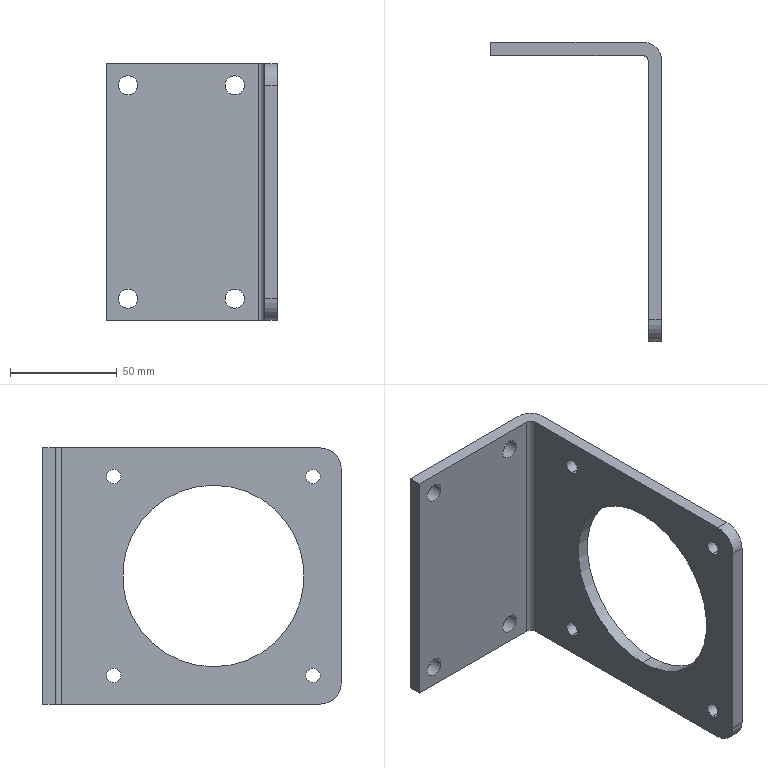Part | STEP file | X77-07004 | 1 solid | 30 faces | box 80 x 140 x 120 mm | volume 115961 mm3 | cylinder 22 | plane 8 | commonest cylinder face diameters 6.8 x8 9 x8 20 x2 85 x2 6 x1 16 x1
STEP:
#1=CARTESIAN_POINT('',(374.189,-142.541,9.95));
#2=VERTEX_POINT('',#1);
#3=CARTESIAN_POINT('',(374.189,-142.541,16.75));
#4=VERTEX_POINT('',#3);
#5=CARTESIAN_POINT('',(374.189,-142.541,13.35));
#6=DIRECTION('',(-1.,0.,0.));
#7=DIRECTION('',(0.,0.,1.));
#8=AXIS2_PLACEMENT_3D('',#5,#6,#7);
#9=CIRCLE('',#8,3.4);
#10=EDGE_CURVE('',#2,#4,#9,.T.);
#11=ORIENTED_EDGE('',*,*,#10,.F.);
#12=CARTESIAN_POINT('',(368.189,-142.541,9.95));
#13=VERTEX_POINT('',#12);
#14=CARTESIAN_POINT('',(368.189,-142.541,9.95));
#15=DIRECTION('',(-1.,0.,0.));
#16=VECTOR('',#15,1000.);
#17=LINE('',#14,#16);
#18=EDGE_CURVE('',#2,#13,#17,.T.);
#19=ORIENTED_EDGE('',*,*,#18,.T.);
#20=CARTESIAN_POINT('',(368.189,-142.541,16.75));
#21=VERTEX_POINT('',#20);
#22=CARTESIAN_POINT('',(368.189,-142.541,13.35));
#23=DIRECTION('',(-1.,0.,0.));
#24=DIRECTION('',(0.,0.,1.));
#25=AXIS2_PLACEMENT_3D('',#22,#23,#24);
#26=CIRCLE('',#25,3.4);
#27=EDGE_CURVE('',#13,#21,#26,.T.);
#28=ORIENTED_EDGE('',*,*,#27,.T.);
#29=CARTESIAN_POINT('',(368.189,-142.541,16.75));
#30=DIRECTION('',(-1.,0.,0.));
#31=VECTOR('',#30,1000.);
#32=LINE('',#29,#31);
#33=EDGE_CURVE('',#4,#21,#32,.T.);
#34=ORIENTED_EDGE('',*,*,#33,.F.);
#35=EDGE_LOOP('',(#11,#19,#28,#34));
#36=FACE_OUTER_BOUND('',#35,.T.);
#37=CARTESIAN_POINT('',(368.189,-142.541,13.35));
#38=DIRECTION('',(-1.,0.,0.));
#39=DIRECTION('',(0.,0.,1.));
#40=AXIS2_PLACEMENT_3D('',#37,#38,#39);
#41=CYLINDRICAL_SURFACE('',#40,3.4);
#42=ADVANCED_FACE('',(#36),#41,.F.);
#43=CARTESIAN_POINT('',(374.189,-142.541,103.25));
#44=VERTEX_POINT('',#43);
#45=CARTESIAN_POINT('',(374.189,-142.541,110.05));
#46=VERTEX_POINT('',#45);
#47=CARTESIAN_POINT('',(374.189,-142.541,106.65));
#48=DIRECTION('',(-1.,0.,0.));
#49=DIRECTION('',(0.,0.,1.));
#50=AXIS2_PLACEMENT_3D('',#47,#48,#49);
#51=CIRCLE('',#50,3.4);
#52=EDGE_CURVE('',#44,#46,#51,.T.);
#53=ORIENTED_EDGE('',*,*,#52,.F.);
#54=CARTESIAN_POINT('',(368.189,-142.541,103.25));
#55=VERTEX_POINT('',#54);
#56=CARTESIAN_POINT('',(368.189,-142.541,103.25));
#57=DIRECTION('',(-1.,0.,0.));
#58=VECTOR('',#57,1000.);
#59=LINE('',#56,#58);
#60=EDGE_CURVE('',#44,#55,#59,.T.);
#61=ORIENTED_EDGE('',*,*,#60,.T.);
#62=CARTESIAN_POINT('',(368.189,-142.541,110.05));
#63=VERTEX_POINT('',#62);
#64=CARTESIAN_POINT('',(368.189,-142.541,106.65));
#65=DIRECTION('',(-1.,0.,0.));
#66=DIRECTION('',(0.,0.,1.));
#67=AXIS2_PLACEMENT_3D('',#64,#65,#66);
#68=CIRCLE('',#67,3.4);
#69=EDGE_CURVE('',#55,#63,#68,.T.);
#70=ORIENTED_EDGE('',*,*,#69,.T.);
#71=CARTESIAN_POINT('',(368.189,-142.541,110.05));
#72=DIRECTION('',(-1.,0.,0.));
#73=VECTOR('',#72,1000.);
#74=LINE('',#71,#73);
#75=EDGE_CURVE('',#46,#63,#74,.T.);
#76=ORIENTED_EDGE('',*,*,#75,.F.);
#77=EDGE_LOOP('',(#53,#61,#70,#76));
#78=FACE_OUTER_BOUND('',#77,.T.);
#79=CARTESIAN_POINT('',(368.189,-142.541,106.65));
#80=DIRECTION('',(-1.,0.,0.));
#81=DIRECTION('',(0.,0.,1.));
#82=AXIS2_PLACEMENT_3D('',#79,#80,#81);
#83=CYLINDRICAL_SURFACE('',#82,3.4);
#84=ADVANCED_FACE('',(#78),#83,.F.);
#85=CARTESIAN_POINT('',(374.189,-49.241,103.25));
#86=VERTEX_POINT('',#85);
#87=CARTESIAN_POINT('',(374.189,-49.241,110.05));
#88=VERTEX_POINT('',#87);
#89=CARTESIAN_POINT('',(374.189,-49.241,106.65));
#90=DIRECTION('',(-1.,0.,0.));
#91=DIRECTION('',(0.,0.,1.));
#92=AXIS2_PLACEMENT_3D('',#89,#90,#91);
#93=CIRCLE('',#92,3.4);
#94=EDGE_CURVE('',#86,#88,#93,.T.);
#95=ORIENTED_EDGE('',*,*,#94,.F.);
#96=CARTESIAN_POINT('',(368.189,-49.241,103.25));
#97=VERTEX_POINT('',#96);
#98=CARTESIAN_POINT('',(368.189,-49.241,103.25));
#99=DIRECTION('',(-1.,0.,0.));
#100=VECTOR('',#99,1000.);
#101=LINE('',#98,#100);
#102=EDGE_CURVE('',#86,#97,#101,.T.);
#103=ORIENTED_EDGE('',*,*,#102,.T.);
#104=CARTESIAN_POINT('',(368.189,-49.241,110.05));
#105=VERTEX_POINT('',#104);
#106=CARTESIAN_POINT('',(368.189,-49.241,106.65));
#107=DIRECTION('',(-1.,0.,0.));
#108=DIRECTION('',(0.,0.,1.));
#109=AXIS2_PLACEMENT_3D('',#106,#107,#108);
#110=CIRCLE('',#109,3.4);
#111=EDGE_CURVE('',#97,#105,#110,.T.);
#112=ORIENTED_EDGE('',*,*,#111,.T.);
#113=CARTESIAN_POINT('',(368.189,-49.241,110.05));
#114=DIRECTION('',(-1.,0.,0.));
#115=VECTOR('',#114,1000.);
#116=LINE('',#113,#115);
#117=EDGE_CURVE('',#88,#105,#116,.T.);
#118=ORIENTED_EDGE('',*,*,#117,.F.);
#119=EDGE_LOOP('',(#95,#103,#112,#118));
#120=FACE_OUTER_BOUND('',#119,.T.);
#121=CARTESIAN_POINT('',(368.189,-49.241,106.65));
#122=DIRECTION('',(-1.,0.,0.));
#123=DIRECTION('',(0.,0.,1.));
#124=AXIS2_PLACEMENT_3D('',#121,#122,#123);
#125=CYLINDRICAL_SURFACE('',#124,3.4);
#126=ADVANCED_FACE('',(#120),#125,.F.);
#127=CARTESIAN_POINT('',(374.189,-49.241,9.95));
#128=VERTEX_POINT('',#127);
#129=CARTESIAN_POINT('',(374.189,-49.241,16.75));
#130=VERTEX_POINT('',#129);
#131=CARTESIAN_POINT('',(374.189,-49.241,13.35));
#132=DIRECTION('',(-1.,0.,0.));
#133=DIRECTION('',(0.,0.,1.));
#134=AXIS2_PLACEMENT_3D('',#131,#132,#133);
#135=CIRCLE('',#134,3.4);
#136=EDGE_CURVE('',#128,#130,#135,.T.);
#137=ORIENTED_EDGE('',*,*,#136,.F.);
#138=CARTESIAN_POINT('',(368.189,-49.241,9.95));
#139=VERTEX_POINT('',#138);
#140=CARTESIAN_POINT('',(368.189,-49.241,9.95));
#141=DIRECTION('',(-1.,0.,0.));
#142=VECTOR('',#141,1000.);
#143=LINE('',#140,#142);
#144=EDGE_CURVE('',#128,#139,#143,.T.);
#145=ORIENTED_EDGE('',*,*,#144,.T.);
#146=CARTESIAN_POINT('',(368.189,-49.241,16.75));
#147=VERTEX_POINT('',#146);
#148=CARTESIAN_POINT('',(368.189,-49.241,13.35));
#149=DIRECTION('',(-1.,0.,0.));
#150=DIRECTION('',(0.,0.,1.));
#151=AXIS2_PLACEMENT_3D('',#148,#149,#150);
#152=CIRCLE('',#151,3.4);
#153=EDGE_CURVE('',#139,#147,#152,.T.);
#154=ORIENTED_EDGE('',*,*,#153,.T.);
#155=CARTESIAN_POINT('',(368.189,-49.241,16.75));
#156=DIRECTION('',(-1.,0.,0.));
#157=VECTOR('',#156,1000.);
#158=LINE('',#155,#157);
#159=EDGE_CURVE('',#130,#147,#158,.T.);
#160=ORIENTED_EDGE('',*,*,#159,.F.);
#161=EDGE_LOOP('',(#137,#145,#154,#160));
#162=FACE_OUTER_BOUND('',#161,.T.);
#163=CARTESIAN_POINT('',(368.189,-49.241,13.35));
#164=DIRECTION('',(-1.,0.,0.));
#165=DIRECTION('',(0.,0.,1.));
#166=AXIS2_PLACEMENT_3D('',#163,#164,#165);
#167=CYLINDRICAL_SURFACE('',#166,3.4);
#168=ADVANCED_FACE('',(#162),#167,.F.);
#169=CARTESIAN_POINT('',(299.689,-15.891,10.));
#170=VERTEX_POINT('',#169);
#171=CARTESIAN_POINT('',(308.689,-15.891,10.));
#172=VERTEX_POINT('',#171);
#173=CARTESIAN_POINT('',(304.189,-15.891,10.));
#174=DIRECTION('',(0.,-1.,0.));
#175=DIRECTION('',(0.,0.,-1.));
#176=AXIS2_PLACEMENT_3D('',#173,#174,#175);
#177=CIRCLE('',#176,4.5);
#178=EDGE_CURVE('',#170,#172,#177,.T.);
#179=ORIENTED_EDGE('',*,*,#178,.F.);
#180=CARTESIAN_POINT('',(299.689,-21.891,10.));
#181=VERTEX_POINT('',#180);
#182=CARTESIAN_POINT('',(299.689,-11.891,10.));
#183=DIRECTION('',(0.,-1.,0.));
#184=VECTOR('',#183,1000.);
#185=LINE('',#182,#184);
#186=EDGE_CURVE('',#170,#181,#185,.T.);
#187=ORIENTED_EDGE('',*,*,#186,.T.);
#188=CARTESIAN_POINT('',(308.689,-21.891,10.));
#189=VERTEX_POINT('',#188);
#190=CARTESIAN_POINT('',(304.189,-21.891,10.));
#191=DIRECTION('',(0.,-1.,0.));
#192=DIRECTION('',(1.,0.,0.));
#193=AXIS2_PLACEMENT_3D('',#190,#191,#192);
#194=CIRCLE('',#193,4.5);
#195=EDGE_CURVE('',#181,#189,#194,.T.);
#196=ORIENTED_EDGE('',*,*,#195,.T.);
#197=CARTESIAN_POINT('',(308.689,-11.891,10.));
#198=DIRECTION('',(0.,-1.,0.));
#199=VECTOR('',#198,1000.);
#200=LINE('',#197,#199);
#201=EDGE_CURVE('',#172,#189,#200,.T.);
#202=ORIENTED_EDGE('',*,*,#201,.F.);
#203=EDGE_LOOP('',(#179,#187,#196,#202));
#204=FACE_OUTER_BOUND('',#203,.T.);
#205=CARTESIAN_POINT('',(304.189,-11.891,10.));
#206=DIRECTION('',(0.,-1.,0.));
#207=DIRECTION('',(1.,0.,0.));
#208=AXIS2_PLACEMENT_3D('',#205,#206,#207);
#209=CYLINDRICAL_SURFACE('',#208,4.5);
#210=ADVANCED_FACE('',(#204),#209,.F.);
#211=CARTESIAN_POINT('',(349.689,-15.891,10.));
#212=VERTEX_POINT('',#211);
#213=CARTESIAN_POINT('',(358.689,-15.891,10.));
#214=VERTEX_POINT('',#213);
#215=CARTESIAN_POINT('',(354.189,-15.891,10.));
#216=DIRECTION('',(0.,-1.,0.));
#217=DIRECTION('',(0.,0.,-1.));
#218=AXIS2_PLACEMENT_3D('',#215,#216,#217);
#219=CIRCLE('',#218,4.5);
#220=EDGE_CURVE('',#212,#214,#219,.T.);
#221=ORIENTED_EDGE('',*,*,#220,.F.);
#222=CARTESIAN_POINT('',(349.689,-21.891,10.));
#223=VERTEX_POINT('',#222);
#224=CARTESIAN_POINT('',(349.689,-11.891,10.));
#225=DIRECTION('',(0.,-1.,0.));
#226=VECTOR('',#225,1000.);
#227=LINE('',#224,#226);
#228=EDGE_CURVE('',#212,#223,#227,.T.);
#229=ORIENTED_EDGE('',*,*,#228,.T.);
#230=CARTESIAN_POINT('',(358.689,-21.891,10.));
#231=VERTEX_POINT('',#230);
#232=CARTESIAN_POINT('',(354.189,-21.891,10.));
#233=DIRECTION('',(0.,-1.,0.));
#234=DIRECTION('',(1.,0.,0.));
#235=AXIS2_PLACEMENT_3D('',#232,#233,#234);
#236=CIRCLE('',#235,4.5);
#237=EDGE_CURVE('',#223,#231,#236,.T.);
#238=ORIENTED_EDGE('',*,*,#237,.T.);
#239=CARTESIAN_POINT('',(358.689,-11.891,10.));
#240=DIRECTION('',(0.,-1.,0.));
#241=VECTOR('',#240,1000.);
#242=LINE('',#239,#241);
#243=EDGE_CURVE('',#214,#231,#242,.T.);
#244=ORIENTED_EDGE('',*,*,#243,.F.);
#245=EDGE_LOOP('',(#221,#229,#238,#244));
#246=FACE_OUTER_BOUND('',#245,.T.);
#247=CARTESIAN_POINT('',(354.189,-11.891,10.));
#248=DIRECTION('',(0.,-1.,0.));
#249=DIRECTION('',(1.,0.,0.));
#250=AXIS2_PLACEMENT_3D('',#247,#248,#249);
#251=CYLINDRICAL_SURFACE('',#250,4.5);
#252=ADVANCED_FACE('',(#246),#251,.F.);
#253=CARTESIAN_POINT('',(349.689,-15.891,110.));
#254=VERTEX_POINT('',#253);
#255=CARTESIAN_POINT('',(358.689,-15.891,110.));
#256=VERTEX_POINT('',#255);
#257=CARTESIAN_POINT('',(354.189,-15.891,110.));
#258=DIRECTION('',(0.,-1.,0.));
#259=DIRECTION('',(0.,0.,-1.));
#260=AXIS2_PLACEMENT_3D('',#257,#258,#259);
#261=CIRCLE('',#260,4.5);
#262=EDGE_CURVE('',#254,#256,#261,.T.);
#263=ORIENTED_EDGE('',*,*,#262,.F.);
#264=CARTESIAN_POINT('',(349.689,-21.891,110.));
#265=VERTEX_POINT('',#264);
#266=CARTESIAN_POINT('',(349.689,-11.891,110.));
#267=DIRECTION('',(0.,-1.,0.));
#268=VECTOR('',#267,1000.);
#269=LINE('',#266,#268);
#270=EDGE_CURVE('',#254,#265,#269,.T.);
#271=ORIENTED_EDGE('',*,*,#270,.T.);
#272=CARTESIAN_POINT('',(358.689,-21.891,110.));
#273=VERTEX_POINT('',#272);
#274=CARTESIAN_POINT('',(354.189,-21.891,110.));
#275=DIRECTION('',(0.,-1.,0.));
#276=DIRECTION('',(1.,0.,0.));
#277=AXIS2_PLACEMENT_3D('',#274,#275,#276);
#278=CIRCLE('',#277,4.5);
#279=EDGE_CURVE('',#265,#273,#278,.T.);
#280=ORIENTED_EDGE('',*,*,#279,.T.);
#281=CARTESIAN_POINT('',(358.689,-11.891,110.));
#282=DIRECTION('',(0.,-1.,0.));
#283=VECTOR('',#282,1000.);
#284=LINE('',#281,#283);
#285=EDGE_CURVE('',#256,#273,#284,.T.);
#286=ORIENTED_EDGE('',*,*,#285,.F.);
#287=EDGE_LOOP('',(#263,#271,#280,#286));
#288=FACE_OUTER_BOUND('',#287,.T.);
#289=CARTESIAN_POINT('',(354.189,-11.891,110.));
#290=DIRECTION('',(0.,-1.,0.));
#291=DIRECTION('',(1.,0.,0.));
#292=AXIS2_PLACEMENT_3D('',#289,#290,#291);
#293=CYLINDRICAL_SURFACE('',#292,4.5);
#294=ADVANCED_FACE('',(#288),#293,.F.);
#295=CARTESIAN_POINT('',(299.689,-15.891,110.));
#296=VERTEX_POINT('',#295);
#297=CARTESIAN_POINT('',(308.689,-15.891,110.));
#298=VERTEX_POINT('',#297);
#299=CARTESIAN_POINT('',(304.189,-15.891,110.));
#300=DIRECTION('',(0.,-1.,0.));
#301=DIRECTION('',(0.,0.,-1.));
#302=AXIS2_PLACEMENT_3D('',#299,#300,#301);
#303=CIRCLE('',#302,4.5);
#304=EDGE_CURVE('',#296,#298,#303,.T.);
#305=ORIENTED_EDGE('',*,*,#304,.F.);
#306=CARTESIAN_POINT('',(299.689,-21.891,110.));
#307=VERTEX_POINT('',#306);
#308=CARTESIAN_POINT('',(299.689,-11.891,110.));
#309=DIRECTION('',(0.,-1.,0.));
#310=VECTOR('',#309,1000.);
#311=LINE('',#308,#310);
#312=EDGE_CURVE('',#296,#307,#311,.T.);
#313=ORIENTED_EDGE('',*,*,#312,.T.);
#314=CARTESIAN_POINT('',(308.689,-21.891,110.));
#315=VERTEX_POINT('',#314);
#316=CARTESIAN_POINT('',(304.189,-21.891,110.));
#317=DIRECTION('',(0.,-1.,0.));
#318=DIRECTION('',(1.,0.,0.));
#319=AXIS2_PLACEMENT_3D('',#316,#317,#318);
#320=CIRCLE('',#319,4.5);
#321=EDGE_CURVE('',#307,#315,#320,.T.);
#322=ORIENTED_EDGE('',*,*,#321,.T.);
#323=CARTESIAN_POINT('',(308.689,-11.891,110.));
#324=DIRECTION('',(0.,-1.,0.));
#325=VECTOR('',#324,1000.);
#326=LINE('',#323,#325);
#327=EDGE_CURVE('',#298,#315,#326,.T.);
#328=ORIENTED_EDGE('',*,*,#327,.F.);
#329=EDGE_LOOP('',(#305,#313,#322,#328));
#330=FACE_OUTER_BOUND('',#329,.T.);
#331=CARTESIAN_POINT('',(304.189,-11.891,110.));
#332=DIRECTION('',(0.,-1.,0.));
#333=DIRECTION('',(1.,0.,0.));
#334=AXIS2_PLACEMENT_3D('',#331,#332,#333);
#335=CYLINDRICAL_SURFACE('',#334,4.5);
#336=ADVANCED_FACE('',(#330),#335,.F.);
#337=CARTESIAN_POINT('',(368.189,-95.891,102.5));
#338=VERTEX_POINT('',#337);
#339=CARTESIAN_POINT('',(368.189,-95.891,17.5));
#340=VERTEX_POINT('',#339);
#341=CARTESIAN_POINT('',(368.189,-95.891,60.));
#342=DIRECTION('',(1.,0.,0.));
#343=DIRECTION('',(0.,0.,-1.));
#344=AXIS2_PLACEMENT_3D('',#341,#342,#343);
#345=CIRCLE('',#344,42.5);
#346=EDGE_CURVE('',#338,#340,#345,.T.);
#347=ORIENTED_EDGE('',*,*,#346,.F.);
#348=CARTESIAN_POINT('',(374.189,-95.891,102.5));
#349=VERTEX_POINT('',#348);
#350=CARTESIAN_POINT('',(364.189,-95.891,102.5));
#351=DIRECTION('',(1.,0.,0.));
#352=VECTOR('',#351,1000.);
#353=LINE('',#350,#352);
#354=EDGE_CURVE('',#338,#349,#353,.T.);
#355=ORIENTED_EDGE('',*,*,#354,.T.);
#356=CARTESIAN_POINT('',(374.189,-95.891,17.5));
#357=VERTEX_POINT('',#356);
#358=CARTESIAN_POINT('',(374.189,-95.891,60.));
#359=DIRECTION('',(1.,0.,0.));
#360=DIRECTION('',(0.,0.,-1.));
#361=AXIS2_PLACEMENT_3D('',#358,#359,#360);
#362=CIRCLE('',#361,42.5);
#363=EDGE_CURVE('',#349,#357,#362,.T.);
#364=ORIENTED_EDGE('',*,*,#363,.T.);
#365=CARTESIAN_POINT('',(364.189,-95.891,17.5));
#366=DIRECTION('',(1.,0.,0.));
#367=VECTOR('',#366,1000.);
#368=LINE('',#365,#367);
#369=EDGE_CURVE('',#340,#357,#368,.T.);
#370=ORIENTED_EDGE('',*,*,#369,.F.);
#371=EDGE_LOOP('',(#347,#355,#364,#370));
#372=FACE_OUTER_BOUND('',#371,.T.);
#373=CARTESIAN_POINT('',(364.189,-95.891,60.));
#374=DIRECTION('',(1.,0.,0.));
#375=DIRECTION('',(0.,0.,-1.));
#376=AXIS2_PLACEMENT_3D('',#373,#374,#375);
#377=CYLINDRICAL_SURFACE('',#376,42.5);
#378=ADVANCED_FACE('',(#372),#377,.F.);
#379=CARTESIAN_POINT('',(368.189,-155.891,110.));
#380=VERTEX_POINT('',#379);
#381=CARTESIAN_POINT('',(368.189,-155.891,10.));
#382=VERTEX_POINT('',#381);
#383=CARTESIAN_POINT('',(368.189,-155.891,120.));
#384=DIRECTION('',(0.,0.,-1.));
#385=VECTOR('',#384,1000.);
#386=LINE('',#383,#385);
#387=EDGE_CURVE('',#380,#382,#386,.T.);
#388=ORIENTED_EDGE('',*,*,#387,.T.);
#389=CARTESIAN_POINT('',(374.189,-155.891,10.));
#390=VERTEX_POINT('',#389);
#391=CARTESIAN_POINT('',(374.189,-155.891,10.));
#392=DIRECTION('',(1.,0.,0.));
#393=VECTOR('',#392,1000.);
#394=LINE('',#391,#393);
#395=EDGE_CURVE('',#382,#390,#394,.T.);
#396=ORIENTED_EDGE('',*,*,#395,.T.);
#397=CARTESIAN_POINT('',(374.189,-155.891,110.));
#398=VERTEX_POINT('',#397);
#399=CARTESIAN_POINT('',(374.189,-155.891,120.));
#400=DIRECTION('',(0.,0.,-1.));
#401=VECTOR('',#400,1000.);
#402=LINE('',#399,#401);
#403=EDGE_CURVE('',#398,#390,#402,.T.);
#404=ORIENTED_EDGE('',*,*,#403,.F.);
#405=CARTESIAN_POINT('',(374.189,-155.891,110.));
#406=DIRECTION('',(-1.,0.,0.));
#407=VECTOR('',#406,1000.);
#408=LINE('',#405,#407);
#409=EDGE_CURVE('',#398,#380,#408,.T.);
#410=ORIENTED_EDGE('',*,*,#409,.T.);
#411=EDGE_LOOP('',(#388,#396,#404,#410));
#412=FACE_OUTER_BOUND('',#411,.T.);
#413=CARTESIAN_POINT('',(374.189,-155.891,120.));
#414=DIRECTION('',(0.,1.,0.));
#415=DIRECTION('',(0.,0.,1.));
#416=AXIS2_PLACEMENT_3D('',#413,#414,#415);
#417=PLANE('',#416);
#418=ADVANCED_FACE('',(#412),#417,.F.);
#419=CARTESIAN_POINT('',(374.189,-142.541,13.35));
#420=DIRECTION('',(-1.,0.,0.));
#421=DIRECTION('',(0.,0.,1.));
#422=AXIS2_PLACEMENT_3D('',#419,#420,#421);
#423=CIRCLE('',#422,3.4);
#424=EDGE_CURVE('',#4,#2,#423,.T.);
#425=ORIENTED_EDGE('',*,*,#424,.T.);
#426=ORIENTED_EDGE('',*,*,#10,.T.);
#427=EDGE_LOOP('',(#425,#426));
#428=FACE_BOUND('',#427,.T.);
#429=CARTESIAN_POINT('',(374.189,-142.541,106.65));
#430=DIRECTION('',(-1.,0.,0.));
#431=DIRECTION('',(0.,0.,1.));
#432=AXIS2_PLACEMENT_3D('',#429,#430,#431);
#433=CIRCLE('',#432,3.4);
#434=EDGE_CURVE('',#46,#44,#433,.T.);
#435=ORIENTED_EDGE('',*,*,#434,.T.);
#436=ORIENTED_EDGE('',*,*,#52,.T.);
#437=EDGE_LOOP('',(#435,#436));
#438=FACE_BOUND('',#437,.T.);
#439=CARTESIAN_POINT('',(374.189,-49.241,106.65));
#440=DIRECTION('',(-1.,0.,0.));
#441=DIRECTION('',(0.,0.,1.));
#442=AXIS2_PLACEMENT_3D('',#439,#440,#441);
#443=CIRCLE('',#442,3.4);
#444=EDGE_CURVE('',#88,#86,#443,.T.);
#445=ORIENTED_EDGE('',*,*,#444,.T.);
#446=ORIENTED_EDGE('',*,*,#94,.T.);
#447=EDGE_LOOP('',(#445,#446));
#448=FACE_BOUND('',#447,.T.);
#449=CARTESIAN_POINT('',(374.189,-49.241,13.35));
#450=DIRECTION('',(-1.,0.,0.));
#451=DIRECTION('',(0.,0.,1.));
#452=AXIS2_PLACEMENT_3D('',#449,#450,#451);
#453=CIRCLE('',#452,3.4);
#454=EDGE_CURVE('',#130,#128,#453,.T.);
#455=ORIENTED_EDGE('',*,*,#454,.T.);
#456=ORIENTED_EDGE('',*,*,#136,.T.);
#457=EDGE_LOOP('',(#455,#456));
#458=FACE_BOUND('',#457,.T.);
#459=CARTESIAN_POINT('',(374.189,-95.891,60.));
#460=DIRECTION('',(1.,0.,0.));
#461=DIRECTION('',(0.,0.,-1.));
#462=AXIS2_PLACEMENT_3D('',#459,#460,#461);
#463=CIRCLE('',#462,42.5);
#464=EDGE_CURVE('',#357,#349,#463,.T.);
#465=ORIENTED_EDGE('',*,*,#464,.F.);
#466=ORIENTED_EDGE('',*,*,#363,.F.);
#467=EDGE_LOOP('',(#465,#466));
#468=FACE_BOUND('',#467,.T.);
#469=ORIENTED_EDGE('',*,*,#403,.T.);
#470=CARTESIAN_POINT('',(374.189,-145.891,0.));
#471=VERTEX_POINT('',#470);
#472=CARTESIAN_POINT('',(374.189,-145.891,10.));
#473=DIRECTION('',(1.,0.,0.));
#474=DIRECTION('',(0.,0.,1.));
#475=AXIS2_PLACEMENT_3D('',#472,#473,#474);
#476=CIRCLE('',#475,10.);
#477=EDGE_CURVE('',#390,#471,#476,.T.);
#478=ORIENTED_EDGE('',*,*,#477,.T.);
#479=CARTESIAN_POINT('',(374.189,-23.891,0.));
#480=VERTEX_POINT('',#479);
#481=CARTESIAN_POINT('',(374.189,-23.891,0.));
#482=DIRECTION('',(0.,1.,0.));
#483=VECTOR('',#482,1000.);
#484=LINE('',#481,#483);
#485=EDGE_CURVE('',#471,#480,#484,.T.);
#486=ORIENTED_EDGE('',*,*,#485,.T.);
#487=CARTESIAN_POINT('',(374.189,-23.891,120.));
#488=VERTEX_POINT('',#487);
#489=CARTESIAN_POINT('',(374.189,-23.891,120.));
#490=DIRECTION('',(0.,0.,-1.));
#491=VECTOR('',#490,1000.);
#492=LINE('',#489,#491);
#493=EDGE_CURVE('',#488,#480,#492,.T.);
#494=ORIENTED_EDGE('',*,*,#493,.F.);
#495=CARTESIAN_POINT('',(374.189,-145.891,120.));
#496=VERTEX_POINT('',#495);
#497=CARTESIAN_POINT('',(374.189,-23.891,120.));
#498=DIRECTION('',(0.,1.,0.));
#499=VECTOR('',#498,1000.);
#500=LINE('',#497,#499);
#501=EDGE_CURVE('',#496,#488,#500,.T.);
#502=ORIENTED_EDGE('',*,*,#501,.F.);
#503=CARTESIAN_POINT('',(374.189,-145.891,110.));
#504=DIRECTION('',(1.,0.,0.));
#505=DIRECTION('',(0.,0.,1.));
#506=AXIS2_PLACEMENT_3D('',#503,#504,#505);
#507=CIRCLE('',#506,10.);
#508=EDGE_CURVE('',#496,#398,#507,.T.);
#509=ORIENTED_EDGE('',*,*,#508,.T.);
#510=EDGE_LOOP('',(#469,#478,#486,#494,#502,#509));
#511=FACE_OUTER_BOUND('',#510,.T.);
#512=CARTESIAN_POINT('',(374.189,-23.891,120.));
#513=DIRECTION('',(-1.,0.,0.));
#514=DIRECTION('',(0.,0.,1.));
#515=AXIS2_PLACEMENT_3D('',#512,#513,#514);
#516=PLANE('',#515);
#517=ADVANCED_FACE('',(#428,#438,#448,#458,#468,#511),#516,.F.);
#518=CARTESIAN_POINT('',(366.189,-15.891,0.));
#519=VERTEX_POINT('',#518);
#520=CARTESIAN_POINT('',(366.189,-23.891,0.));
#521=DIRECTION('',(0.,0.,1.));
#522=DIRECTION('',(-1.,0.,0.));
#523=AXIS2_PLACEMENT_3D('',#520,#521,#522);
#524=CIRCLE('',#523,8.);
#525=EDGE_CURVE('',#480,#519,#524,.T.);
#526=ORIENTED_EDGE('',*,*,#525,.T.);
#527=CARTESIAN_POINT('',(366.189,-15.891,120.));
#528=VERTEX_POINT('',#527);
#529=CARTESIAN_POINT('',(366.189,-15.891,120.));
#530=DIRECTION('',(0.,0.,-1.));
#531=VECTOR('',#530,1000.);
#532=LINE('',#529,#531);
#533=EDGE_CURVE('',#528,#519,#532,.T.);
#534=ORIENTED_EDGE('',*,*,#533,.F.);
#535=CARTESIAN_POINT('',(366.189,-23.891,120.));
#536=DIRECTION('',(0.,0.,1.));
#537=DIRECTION('',(-1.,0.,0.));
#538=AXIS2_PLACEMENT_3D('',#535,#536,#537);
#539=CIRCLE('',#538,8.);
#540=EDGE_CURVE('',#488,#528,#539,.T.);
#541=ORIENTED_EDGE('',*,*,#540,.F.);
#542=ORIENTED_EDGE('',*,*,#493,.T.);
#543=EDGE_LOOP('',(#526,#534,#541,#542));
#544=FACE_OUTER_BOUND('',#543,.T.);
#545=CARTESIAN_POINT('',(366.189,-23.891,120.));
#546=DIRECTION('',(0.,0.,-1.));
#547=DIRECTION('',(-1.,0.,0.));
#548=AXIS2_PLACEMENT_3D('',#545,#546,#547);
#549=CYLINDRICAL_SURFACE('',#548,8.);
#550=ADVANCED_FACE('',(#544),#549,.T.);
#551=CARTESIAN_POINT('',(304.189,-15.891,10.));
#552=DIRECTION('',(0.,-1.,0.));
#553=DIRECTION('',(0.,0.,-1.));
#554=AXIS2_PLACEMENT_3D('',#551,#552,#553);
#555=CIRCLE('',#554,4.5);
#556=EDGE_CURVE('',#172,#170,#555,.T.);
#557=ORIENTED_EDGE('',*,*,#556,.T.);
#558=ORIENTED_EDGE('',*,*,#178,.T.);
#559=EDGE_LOOP('',(#557,#558));
#560=FACE_BOUND('',#559,.T.);
#561=CARTESIAN_POINT('',(354.189,-15.891,10.));
#562=DIRECTION('',(0.,-1.,0.));
#563=DIRECTION('',(0.,0.,-1.));
#564=AXIS2_PLACEMENT_3D('',#561,#562,#563);
#565=CIRCLE('',#564,4.5);
#566=EDGE_CURVE('',#214,#212,#565,.T.);
#567=ORIENTED_EDGE('',*,*,#566,.T.);
#568=ORIENTED_EDGE('',*,*,#220,.T.);
#569=EDGE_LOOP('',(#567,#568));
#570=FACE_BOUND('',#569,.T.);
#571=CARTESIAN_POINT('',(354.189,-15.891,110.));
#572=DIRECTION('',(0.,-1.,0.));
#573=DIRECTION('',(0.,0.,-1.));
#574=AXIS2_PLACEMENT_3D('',#571,#572,#573);
#575=CIRCLE('',#574,4.5);
#576=EDGE_CURVE('',#256,#254,#575,.T.);
#577=ORIENTED_EDGE('',*,*,#576,.T.);
#578=ORIENTED_EDGE('',*,*,#262,.T.);
#579=EDGE_LOOP('',(#577,#578));
#580=FACE_BOUND('',#579,.T.);
#581=CARTESIAN_POINT('',(304.189,-15.891,110.));
#582=DIRECTION('',(0.,-1.,0.));
#583=DIRECTION('',(0.,0.,-1.));
#584=AXIS2_PLACEMENT_3D('',#581,#582,#583);
#585=CIRCLE('',#584,4.5);
#586=EDGE_CURVE('',#298,#296,#585,.T.);
#587=ORIENTED_EDGE('',*,*,#586,.T.);
#588=ORIENTED_EDGE('',*,*,#304,.T.);
#589=EDGE_LOOP('',(#587,#588));
#590=FACE_BOUND('',#589,.T.);
#591=CARTESIAN_POINT('',(294.189,-15.891,0.));
#592=VERTEX_POINT('',#591);
#593=CARTESIAN_POINT('',(294.189,-15.891,0.));
#594=DIRECTION('',(-1.,0.,0.));
#595=VECTOR('',#594,1000.);
#596=LINE('',#593,#595);
#597=EDGE_CURVE('',#519,#592,#596,.T.);
#598=ORIENTED_EDGE('',*,*,#597,.T.);
#599=CARTESIAN_POINT('',(294.189,-15.891,120.));
#600=VERTEX_POINT('',#599);
#601=CARTESIAN_POINT('',(294.189,-15.891,120.));
#602=DIRECTION('',(0.,0.,-1.));
#603=VECTOR('',#602,1000.);
#604=LINE('',#601,#603);
#605=EDGE_CURVE('',#600,#592,#604,.T.);
#606=ORIENTED_EDGE('',*,*,#605,.F.);
#607=CARTESIAN_POINT('',(294.189,-15.891,120.));
#608=DIRECTION('',(-1.,0.,0.));
#609=VECTOR('',#608,1000.);
#610=LINE('',#607,#609);
#611=EDGE_CURVE('',#528,#600,#610,.T.);
#612=ORIENTED_EDGE('',*,*,#611,.F.);
#613=ORIENTED_EDGE('',*,*,#533,.T.);
#614=EDGE_LOOP('',(#598,#606,#612,#613));
#615=FACE_OUTER_BOUND('',#614,.T.);
#616=CARTESIAN_POINT('',(294.189,-15.891,120.));
#617=DIRECTION('',(0.,-1.,0.));
#618=DIRECTION('',(0.,0.,-1.));
#619=AXIS2_PLACEMENT_3D('',#616,#617,#618);
#620=PLANE('',#619);
#621=ADVANCED_FACE('',(#560,#570,#580,#590,#615),#620,.F.);
#622=CARTESIAN_POINT('',(294.189,-21.891,0.));
#623=VERTEX_POINT('',#622);
#624=CARTESIAN_POINT('',(294.189,-21.891,0.));
#625=DIRECTION('',(0.,-1.,0.));
#626=VECTOR('',#625,1000.);
#627=LINE('',#624,#626);
#628=EDGE_CURVE('',#592,#623,#627,.T.);
#629=ORIENTED_EDGE('',*,*,#628,.T.);
#630=CARTESIAN_POINT('',(294.189,-21.891,120.));
#631=VERTEX_POINT('',#630);
#632=CARTESIAN_POINT('',(294.189,-21.891,120.));
#633=DIRECTION('',(0.,0.,-1.));
#634=VECTOR('',#633,1000.);
#635=LINE('',#632,#634);
#636=EDGE_CURVE('',#631,#623,#635,.T.);
#637=ORIENTED_EDGE('',*,*,#636,.F.);
#638=CARTESIAN_POINT('',(294.189,-21.891,120.));
#639=DIRECTION('',(0.,-1.,0.));
#640=VECTOR('',#639,1000.);
#641=LINE('',#638,#640);
#642=EDGE_CURVE('',#600,#631,#641,.T.);
#643=ORIENTED_EDGE('',*,*,#642,.F.);
#644=ORIENTED_EDGE('',*,*,#605,.T.);
#645=EDGE_LOOP('',(#629,#637,#643,#644));
#646=FACE_OUTER_BOUND('',#645,.T.);
#647=CARTESIAN_POINT('',(294.189,-21.891,120.));
#648=DIRECTION('',(1.,0.,0.));
#649=DIRECTION('',(0.,0.,-1.));
#650=AXIS2_PLACEMENT_3D('',#647,#648,#649);
#651=PLANE('',#650);
#652=ADVANCED_FACE('',(#646),#651,.F.);
#653=CARTESIAN_POINT('',(304.189,-21.891,10.));
#654=DIRECTION('',(0.,-1.,0.));
#655=DIRECTION('',(1.,0.,0.));
#656=AXIS2_PLACEMENT_3D('',#653,#654,#655);
#657=CIRCLE('',#656,4.5);
#658=EDGE_CURVE('',#189,#181,#657,.T.);
#659=ORIENTED_EDGE('',*,*,#658,.F.);
#660=ORIENTED_EDGE('',*,*,#195,.F.);
#661=EDGE_LOOP('',(#659,#660));
#662=FACE_BOUND('',#661,.T.);
#663=CARTESIAN_POINT('',(354.189,-21.891,10.));
#664=DIRECTION('',(0.,-1.,0.));
#665=DIRECTION('',(1.,0.,0.));
#666=AXIS2_PLACEMENT_3D('',#663,#664,#665);
#667=CIRCLE('',#666,4.5);
#668=EDGE_CURVE('',#231,#223,#667,.T.);
#669=ORIENTED_EDGE('',*,*,#668,.F.);
#670=ORIENTED_EDGE('',*,*,#237,.F.);
#671=EDGE_LOOP('',(#669,#670));
#672=FACE_BOUND('',#671,.T.);
#673=CARTESIAN_POINT('',(354.189,-21.891,110.));
#674=DIRECTION('',(0.,-1.,0.));
#675=DIRECTION('',(1.,0.,0.));
#676=AXIS2_PLACEMENT_3D('',#673,#674,#675);
#677=CIRCLE('',#676,4.5);
#678=EDGE_CURVE('',#273,#265,#677,.T.);
#679=ORIENTED_EDGE('',*,*,#678,.F.);
#680=ORIENTED_EDGE('',*,*,#279,.F.);
#681=EDGE_LOOP('',(#679,#680));
#682=FACE_BOUND('',#681,.T.);
#683=CARTESIAN_POINT('',(304.189,-21.891,110.));
#684=DIRECTION('',(0.,-1.,0.));
#685=DIRECTION('',(1.,0.,0.));
#686=AXIS2_PLACEMENT_3D('',#683,#684,#685);
#687=CIRCLE('',#686,4.5);
#688=EDGE_CURVE('',#315,#307,#687,.T.);
#689=ORIENTED_EDGE('',*,*,#688,.F.);
#690=ORIENTED_EDGE('',*,*,#321,.F.);
#691=EDGE_LOOP('',(#689,#690));
#692=FACE_BOUND('',#691,.T.);
#693=CARTESIAN_POINT('',(365.189,-21.891,0.));
#694=VERTEX_POINT('',#693);
#695=CARTESIAN_POINT('',(365.189,-21.891,0.));
#696=DIRECTION('',(1.,0.,0.));
#697=VECTOR('',#696,1000.);
#698=LINE('',#695,#697);
#699=EDGE_CURVE('',#623,#694,#698,.T.);
#700=ORIENTED_EDGE('',*,*,#699,.T.);
#701=CARTESIAN_POINT('',(365.189,-21.891,120.));
#702=VERTEX_POINT('',#701);
#703=CARTESIAN_POINT('',(365.189,-21.891,120.));
#704=DIRECTION('',(0.,0.,-1.));
#705=VECTOR('',#704,1000.);
#706=LINE('',#703,#705);
#707=EDGE_CURVE('',#702,#694,#706,.T.);
#708=ORIENTED_EDGE('',*,*,#707,.F.);
#709=CARTESIAN_POINT('',(365.189,-21.891,120.));
#710=DIRECTION('',(1.,0.,0.));
#711=VECTOR('',#710,1000.);
#712=LINE('',#709,#711);
#713=EDGE_CURVE('',#631,#702,#712,.T.);
#714=ORIENTED_EDGE('',*,*,#713,.F.);
#715=ORIENTED_EDGE('',*,*,#636,.T.);
#716=EDGE_LOOP('',(#700,#708,#714,#715));
#717=FACE_OUTER_BOUND('',#716,.T.);
#718=CARTESIAN_POINT('',(365.189,-21.891,120.));
#719=DIRECTION('',(0.,1.,0.));
#720=DIRECTION('',(-1.,0.,0.));
#721=AXIS2_PLACEMENT_3D('',#718,#719,#720);
#722=PLANE('',#721);
#723=ADVANCED_FACE('',(#662,#672,#682,#692,#717),#722,.F.);
#724=CARTESIAN_POINT('',(368.189,-24.891,0.));
#725=VERTEX_POINT('',#724);
#726=CARTESIAN_POINT('',(365.189,-24.891,0.));
#727=DIRECTION('',(0.,0.,-1.));
#728=DIRECTION('',(-1.,0.,0.));
#729=AXIS2_PLACEMENT_3D('',#726,#727,#728);
#730=CIRCLE('',#729,3.);
#731=EDGE_CURVE('',#694,#725,#730,.T.);
#732=ORIENTED_EDGE('',*,*,#731,.T.);
#733=CARTESIAN_POINT('',(368.189,-24.891,120.));
#734=VERTEX_POINT('',#733);
#735=CARTESIAN_POINT('',(368.189,-24.891,120.));
#736=DIRECTION('',(0.,0.,-1.));
#737=VECTOR('',#736,1000.);
#738=LINE('',#735,#737);
#739=EDGE_CURVE('',#734,#725,#738,.T.);
#740=ORIENTED_EDGE('',*,*,#739,.F.);
#741=CARTESIAN_POINT('',(365.189,-24.891,120.));
#742=DIRECTION('',(0.,0.,-1.));
#743=DIRECTION('',(-1.,0.,0.));
#744=AXIS2_PLACEMENT_3D('',#741,#742,#743);
#745=CIRCLE('',#744,3.);
#746=EDGE_CURVE('',#702,#734,#745,.T.);
#747=ORIENTED_EDGE('',*,*,#746,.F.);
#748=ORIENTED_EDGE('',*,*,#707,.T.);
#749=EDGE_LOOP('',(#732,#740,#747,#748));
#750=FACE_OUTER_BOUND('',#749,.T.);
#751=CARTESIAN_POINT('',(365.189,-24.891,120.));
#752=DIRECTION('',(0.,0.,-1.));
#753=DIRECTION('',(-1.,0.,0.));
#754=AXIS2_PLACEMENT_3D('',#751,#752,#753);
#755=CYLINDRICAL_SURFACE('',#754,3.);
#756=ADVANCED_FACE('',(#750),#755,.F.);
#757=CARTESIAN_POINT('',(368.189,-142.541,13.35));
#758=DIRECTION('',(-1.,0.,0.));
#759=DIRECTION('',(0.,0.,1.));
#760=AXIS2_PLACEMENT_3D('',#757,#758,#759);
#761=CIRCLE('',#760,3.4);
#762=EDGE_CURVE('',#21,#13,#761,.T.);
#763=ORIENTED_EDGE('',*,*,#762,.F.);
#764=ORIENTED_EDGE('',*,*,#27,.F.);
#765=EDGE_LOOP('',(#763,#764));
#766=FACE_BOUND('',#765,.T.);
#767=CARTESIAN_POINT('',(368.189,-142.541,106.65));
#768=DIRECTION('',(-1.,0.,0.));
#769=DIRECTION('',(0.,0.,1.));
#770=AXIS2_PLACEMENT_3D('',#767,#768,#769);
#771=CIRCLE('',#770,3.4);
#772=EDGE_CURVE('',#63,#55,#771,.T.);
#773=ORIENTED_EDGE('',*,*,#772,.F.);
#774=ORIENTED_EDGE('',*,*,#69,.F.);
#775=EDGE_LOOP('',(#773,#774));
#776=FACE_BOUND('',#775,.T.);
#777=CARTESIAN_POINT('',(368.189,-49.241,106.65));
#778=DIRECTION('',(-1.,0.,0.));
#779=DIRECTION('',(0.,0.,1.));
#780=AXIS2_PLACEMENT_3D('',#777,#778,#779);
#781=CIRCLE('',#780,3.4);
#782=EDGE_CURVE('',#105,#97,#781,.T.);
#783=ORIENTED_EDGE('',*,*,#782,.F.);
#784=ORIENTED_EDGE('',*,*,#111,.F.);
#785=EDGE_LOOP('',(#783,#784));
#786=FACE_BOUND('',#785,.T.);
#787=CARTESIAN_POINT('',(368.189,-49.241,13.35));
#788=DIRECTION('',(-1.,0.,0.));
#789=DIRECTION('',(0.,0.,1.));
#790=AXIS2_PLACEMENT_3D('',#787,#788,#789);
#791=CIRCLE('',#790,3.4);
#792=EDGE_CURVE('',#147,#139,#791,.T.);
#793=ORIENTED_EDGE('',*,*,#792,.F.);
#794=ORIENTED_EDGE('',*,*,#153,.F.);
#795=EDGE_LOOP('',(#793,#794));
#796=FACE_BOUND('',#795,.T.);
#797=CARTESIAN_POINT('',(368.189,-95.891,60.));
#798=DIRECTION('',(1.,0.,0.));
#799=DIRECTION('',(0.,0.,-1.));
#800=AXIS2_PLACEMENT_3D('',#797,#798,#799);
#801=CIRCLE('',#800,42.5);
#802=EDGE_CURVE('',#340,#338,#801,.T.);
#803=ORIENTED_EDGE('',*,*,#802,.T.);
#804=ORIENTED_EDGE('',*,*,#346,.T.);
#805=EDGE_LOOP('',(#803,#804));
#806=FACE_BOUND('',#805,.T.);
#807=CARTESIAN_POINT('',(368.189,-145.891,0.));
#808=VERTEX_POINT('',#807);
#809=CARTESIAN_POINT('',(368.189,-155.891,0.));
#810=DIRECTION('',(0.,-1.,0.));
#811=VECTOR('',#810,1000.);
#812=LINE('',#809,#811);
#813=EDGE_CURVE('',#725,#808,#812,.T.);
#814=ORIENTED_EDGE('',*,*,#813,.T.);
#815=CARTESIAN_POINT('',(368.189,-145.891,10.));
#816=DIRECTION('',(-1.,0.,0.));
#817=DIRECTION('',(0.,0.,-1.));
#818=AXIS2_PLACEMENT_3D('',#815,#816,#817);
#819=CIRCLE('',#818,10.);
#820=EDGE_CURVE('',#808,#382,#819,.T.);
#821=ORIENTED_EDGE('',*,*,#820,.T.);
#822=ORIENTED_EDGE('',*,*,#387,.F.);
#823=CARTESIAN_POINT('',(368.189,-145.891,120.));
#824=VERTEX_POINT('',#823);
#825=CARTESIAN_POINT('',(368.189,-145.891,110.));
#826=DIRECTION('',(-1.,0.,0.));
#827=DIRECTION('',(0.,0.,-1.));
#828=AXIS2_PLACEMENT_3D('',#825,#826,#827);
#829=CIRCLE('',#828,10.);
#830=EDGE_CURVE('',#380,#824,#829,.T.);
#831=ORIENTED_EDGE('',*,*,#830,.T.);
#832=CARTESIAN_POINT('',(368.189,-155.891,120.));
#833=DIRECTION('',(0.,-1.,0.));
#834=VECTOR('',#833,1000.);
#835=LINE('',#832,#834);
#836=EDGE_CURVE('',#734,#824,#835,.T.);
#837=ORIENTED_EDGE('',*,*,#836,.F.);
#838=ORIENTED_EDGE('',*,*,#739,.T.);
#839=EDGE_LOOP('',(#814,#821,#822,#831,#837,#838));
#840=FACE_OUTER_BOUND('',#839,.T.);
#841=CARTESIAN_POINT('',(368.189,-155.891,120.));
#842=DIRECTION('',(1.,0.,0.));
#843=DIRECTION('',(0.,0.,-1.));
#844=AXIS2_PLACEMENT_3D('',#841,#842,#843);
#845=PLANE('',#844);
#846=ADVANCED_FACE('',(#766,#776,#786,#796,#806,#840),#845,.F.);
#847=ORIENTED_EDGE('',*,*,#836,.T.);
#848=CARTESIAN_POINT('',(365.189,-145.891,120.));
#849=DIRECTION('',(1.,0.,0.));
#850=VECTOR('',#849,1000.);
#851=LINE('',#848,#850);
#852=EDGE_CURVE('',#824,#496,#851,.T.);
#853=ORIENTED_EDGE('',*,*,#852,.T.);
#854=ORIENTED_EDGE('',*,*,#501,.T.);
#855=ORIENTED_EDGE('',*,*,#540,.T.);
#856=ORIENTED_EDGE('',*,*,#611,.T.);
#857=ORIENTED_EDGE('',*,*,#642,.T.);
#858=ORIENTED_EDGE('',*,*,#713,.T.);
#859=ORIENTED_EDGE('',*,*,#746,.T.);
#860=EDGE_LOOP('',(#847,#853,#854,#855,#856,#857,#858,#859));
#861=FACE_OUTER_BOUND('',#860,.T.);
#862=CARTESIAN_POINT('',(365.189,-24.891,120.));
#863=DIRECTION('',(0.,0.,-1.));
#864=DIRECTION('',(-1.,0.,0.));
#865=AXIS2_PLACEMENT_3D('',#862,#863,#864);
#866=PLANE('',#865);
#867=ADVANCED_FACE('',(#861),#866,.F.);
#868=ORIENTED_EDGE('',*,*,#485,.F.);
#869=CARTESIAN_POINT('',(368.189,-145.891,0.));
#870=DIRECTION('',(-1.,0.,0.));
#871=VECTOR('',#870,1000.);
#872=LINE('',#869,#871);
#873=EDGE_CURVE('',#471,#808,#872,.T.);
#874=ORIENTED_EDGE('',*,*,#873,.T.);
#875=ORIENTED_EDGE('',*,*,#813,.F.);
#876=ORIENTED_EDGE('',*,*,#731,.F.);
#877=ORIENTED_EDGE('',*,*,#699,.F.);
#878=ORIENTED_EDGE('',*,*,#628,.F.);
#879=ORIENTED_EDGE('',*,*,#597,.F.);
#880=ORIENTED_EDGE('',*,*,#525,.F.);
#881=EDGE_LOOP('',(#868,#874,#875,#876,#877,#878,#879,#880));
#882=FACE_OUTER_BOUND('',#881,.T.);
#883=CARTESIAN_POINT('',(365.189,-24.891,0.));
#884=DIRECTION('',(0.,0.,-1.));
#885=DIRECTION('',(-1.,0.,0.));
#886=AXIS2_PLACEMENT_3D('',#883,#884,#885);
#887=PLANE('',#886);
#888=ADVANCED_FACE('',(#882),#887,.T.);
#889=ORIENTED_EDGE('',*,*,#354,.F.);
#890=ORIENTED_EDGE('',*,*,#802,.F.);
#891=ORIENTED_EDGE('',*,*,#369,.T.);
#892=ORIENTED_EDGE('',*,*,#464,.T.);
#893=EDGE_LOOP('',(#889,#890,#891,#892));
#894=FACE_OUTER_BOUND('',#893,.T.);
#895=CARTESIAN_POINT('',(364.189,-95.891,60.));
#896=DIRECTION('',(1.,0.,0.));
#897=DIRECTION('',(0.,0.,-1.));
#898=AXIS2_PLACEMENT_3D('',#895,#896,#897);
#899=CYLINDRICAL_SURFACE('',#898,42.5);
#900=ADVANCED_FACE('',(#894),#899,.F.);
#901=ORIENTED_EDGE('',*,*,#820,.F.);
#902=ORIENTED_EDGE('',*,*,#873,.F.);
#903=ORIENTED_EDGE('',*,*,#477,.F.);
#904=ORIENTED_EDGE('',*,*,#395,.F.);
#905=EDGE_LOOP('',(#901,#902,#903,#904));
#906=FACE_OUTER_BOUND('',#905,.T.);
#907=CARTESIAN_POINT('',(374.189,-145.891,10.));
#908=DIRECTION('',(-1.,0.,0.));
#909=DIRECTION('',(0.,0.,1.));
#910=AXIS2_PLACEMENT_3D('',#907,#908,#909);
#911=CYLINDRICAL_SURFACE('',#910,10.);
#912=ADVANCED_FACE('',(#906),#911,.T.);
#913=ORIENTED_EDGE('',*,*,#830,.F.);
#914=ORIENTED_EDGE('',*,*,#409,.F.);
#915=ORIENTED_EDGE('',*,*,#508,.F.);
#916=ORIENTED_EDGE('',*,*,#852,.F.);
#917=EDGE_LOOP('',(#913,#914,#915,#916));
#918=FACE_OUTER_BOUND('',#917,.T.);
#919=CARTESIAN_POINT('',(365.189,-145.891,110.));
#920=DIRECTION('',(1.,0.,0.));
#921=DIRECTION('',(0.,0.,-1.));
#922=AXIS2_PLACEMENT_3D('',#919,#920,#921);
#923=CYLINDRICAL_SURFACE('',#922,10.);
#924=ADVANCED_FACE('',(#918),#923,.T.);
#925=ORIENTED_EDGE('',*,*,#312,.F.);
#926=ORIENTED_EDGE('',*,*,#586,.F.);
#927=ORIENTED_EDGE('',*,*,#327,.T.);
#928=ORIENTED_EDGE('',*,*,#688,.T.);
#929=EDGE_LOOP('',(#925,#926,#927,#928));
#930=FACE_OUTER_BOUND('',#929,.T.);
#931=CARTESIAN_POINT('',(304.189,-11.891,110.));
#932=DIRECTION('',(0.,-1.,0.));
#933=DIRECTION('',(1.,0.,0.));
#934=AXIS2_PLACEMENT_3D('',#931,#932,#933);
#935=CYLINDRICAL_SURFACE('',#934,4.5);
#936=ADVANCED_FACE('',(#930),#935,.F.);
#937=ORIENTED_EDGE('',*,*,#270,.F.);
#938=ORIENTED_EDGE('',*,*,#576,.F.);
#939=ORIENTED_EDGE('',*,*,#285,.T.);
#940=ORIENTED_EDGE('',*,*,#678,.T.);
#941=EDGE_LOOP('',(#937,#938,#939,#940));
#942=FACE_OUTER_BOUND('',#941,.T.);
#943=CARTESIAN_POINT('',(354.189,-11.891,110.));
#944=DIRECTION('',(0.,-1.,0.));
#945=DIRECTION('',(1.,0.,0.));
#946=AXIS2_PLACEMENT_3D('',#943,#944,#945);
#947=CYLINDRICAL_SURFACE('',#946,4.5);
#948=ADVANCED_FACE('',(#942),#947,.F.);
#949=ORIENTED_EDGE('',*,*,#228,.F.);
#950=ORIENTED_EDGE('',*,*,#566,.F.);
#951=ORIENTED_EDGE('',*,*,#243,.T.);
#952=ORIENTED_EDGE('',*,*,#668,.T.);
#953=EDGE_LOOP('',(#949,#950,#951,#952));
#954=FACE_OUTER_BOUND('',#953,.T.);
#955=CARTESIAN_POINT('',(354.189,-11.891,10.));
#956=DIRECTION('',(0.,-1.,0.));
#957=DIRECTION('',(1.,0.,0.));
#958=AXIS2_PLACEMENT_3D('',#955,#956,#957);
#959=CYLINDRICAL_SURFACE('',#958,4.5);
#960=ADVANCED_FACE('',(#954),#959,.F.);
#961=ORIENTED_EDGE('',*,*,#186,.F.);
#962=ORIENTED_EDGE('',*,*,#556,.F.);
#963=ORIENTED_EDGE('',*,*,#201,.T.);
#964=ORIENTED_EDGE('',*,*,#658,.T.);
#965=EDGE_LOOP('',(#961,#962,#963,#964));
#966=FACE_OUTER_BOUND('',#965,.T.);
#967=CARTESIAN_POINT('',(304.189,-11.891,10.));
#968=DIRECTION('',(0.,-1.,0.));
#969=DIRECTION('',(1.,0.,0.));
#970=AXIS2_PLACEMENT_3D('',#967,#968,#969);
#971=CYLINDRICAL_SURFACE('',#970,4.5);
#972=ADVANCED_FACE('',(#966),#971,.F.);
#973=ORIENTED_EDGE('',*,*,#144,.F.);
#974=ORIENTED_EDGE('',*,*,#454,.F.);
#975=ORIENTED_EDGE('',*,*,#159,.T.);
#976=ORIENTED_EDGE('',*,*,#792,.T.);
#977=EDGE_LOOP('',(#973,#974,#975,#976));
#978=FACE_OUTER_BOUND('',#977,.T.);
#979=CARTESIAN_POINT('',(368.189,-49.241,13.35));
#980=DIRECTION('',(-1.,0.,0.));
#981=DIRECTION('',(0.,0.,1.));
#982=AXIS2_PLACEMENT_3D('',#979,#980,#981);
#983=CYLINDRICAL_SURFACE('',#982,3.4);
#984=ADVANCED_FACE('',(#978),#983,.F.);
#985=ORIENTED_EDGE('',*,*,#102,.F.);
#986=ORIENTED_EDGE('',*,*,#444,.F.);
#987=ORIENTED_EDGE('',*,*,#117,.T.);
#988=ORIENTED_EDGE('',*,*,#782,.T.);
#989=EDGE_LOOP('',(#985,#986,#987,#988));
#990=FACE_OUTER_BOUND('',#989,.T.);
#991=CARTESIAN_POINT('',(368.189,-49.241,106.65));
#992=DIRECTION('',(-1.,0.,0.));
#993=DIRECTION('',(0.,0.,1.));
#994=AXIS2_PLACEMENT_3D('',#991,#992,#993);
#995=CYLINDRICAL_SURFACE('',#994,3.4);
#996=ADVANCED_FACE('',(#990),#995,.F.);
#997=ORIENTED_EDGE('',*,*,#60,.F.);
#998=ORIENTED_EDGE('',*,*,#434,.F.);
#999=ORIENTED_EDGE('',*,*,#75,.T.);
#1000=ORIENTED_EDGE('',*,*,#772,.T.);
#1001=EDGE_LOOP('',(#997,#998,#999,#1000));
#1002=FACE_OUTER_BOUND('',#1001,.T.);
#1003=CARTESIAN_POINT('',(368.189,-142.541,106.65));
#1004=DIRECTION('',(-1.,0.,0.));
#1005=DIRECTION('',(0.,0.,1.));
#1006=AXIS2_PLACEMENT_3D('',#1003,#1004,#1005);
#1007=CYLINDRICAL_SURFACE('',#1006,3.4);
#1008=ADVANCED_FACE('',(#1002),#1007,.F.);
#1009=ORIENTED_EDGE('',*,*,#18,.F.);
#1010=ORIENTED_EDGE('',*,*,#424,.F.);
#1011=ORIENTED_EDGE('',*,*,#33,.T.);
#1012=ORIENTED_EDGE('',*,*,#762,.T.);
#1013=EDGE_LOOP('',(#1009,#1010,#1011,#1012));
#1014=FACE_OUTER_BOUND('',#1013,.T.);
#1015=CARTESIAN_POINT('',(368.189,-142.541,13.35));
#1016=DIRECTION('',(-1.,0.,0.));
#1017=DIRECTION('',(0.,0.,1.));
#1018=AXIS2_PLACEMENT_3D('',#1015,#1016,#1017);
#1019=CYLINDRICAL_SURFACE('',#1018,3.4);
#1020=ADVANCED_FACE('',(#1014),#1019,.F.);
#1021=CLOSED_SHELL('',(#42,#84,#126,#168,#210,#252,#294,#336,#378,#418,#517,#550,#621,#652,#723,#756,#846,#867,#888,#900,#912,#924,#936,#948,#960,#972,#984,#996,#1008,#1020));
#1022=MANIFOLD_SOLID_BREP('',#1021);
#1023=CARTESIAN_POINT('',(0.,0.,0.));
#1024=DIRECTION('',(0.,0.,1.));
#1025=DIRECTION('',(1.,0.,0.));
#1026=AXIS2_PLACEMENT_3D('',#1023,#1024,#1025);
#1027=(LENGTH_UNIT()NAMED_UNIT(*)SI_UNIT(.MILLI.,.METRE.));
#1028=UNCERTAINTY_MEASURE_WITH_UNIT(LENGTH_MEASURE(0.00001),#1027,'','');
#1029=(NAMED_UNIT(*)PLANE_ANGLE_UNIT()SI_UNIT($,.RADIAN.));
#1030=(NAMED_UNIT(*)SI_UNIT($,.STERADIAN.)SOLID_ANGLE_UNIT());
#1031=(GEOMETRIC_REPRESENTATION_CONTEXT(3)GLOBAL_UNCERTAINTY_ASSIGNED_CONTEXT((#1028))GLOBAL_UNIT_ASSIGNED_CONTEXT((#1027,#1029,#1030))REPRESENTATION_CONTEXT('',''));
#1032=ADVANCED_BREP_SHAPE_REPRESENTATION('',(#1022,#1026),#1031);